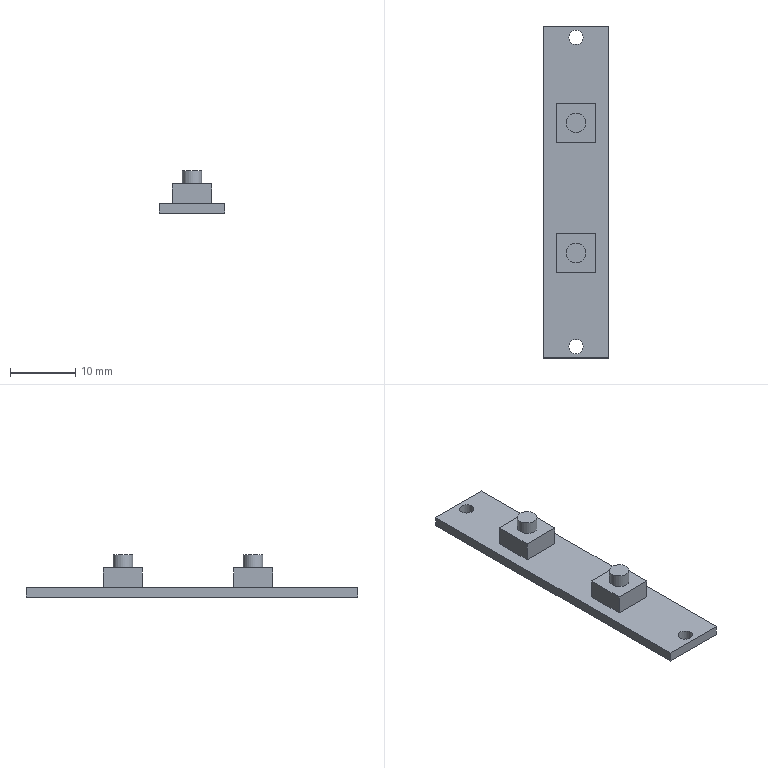Part | STEP file | 1 solid | 22 faces | box 10 x 51 x 6.5 mm | volume 997.87 mm3 | plane 18 | cylinder 4 | commonest cylinder face diameters 2.2 x2 3 x2
STEP:
#1=CARTESIAN_POINT('',(0.,0.,0.));
#2=DIRECTION('',(0.,0.,1.));
#3=DIRECTION('',(1.,0.,0.));
#4=AXIS2_PLACEMENT_3D('',#1,#2,#3);
#5=CARTESIAN_POINT('',(-1.1,12.071,0.));
#6=VERTEX_POINT('',#5);
#7=CARTESIAN_POINT('',(0.,12.071,0.));
#8=DIRECTION('',(0.,0.,-1.));
#9=DIRECTION('',(-1.,0.,0.));
#10=AXIS2_PLACEMENT_3D('',#7,#8,#9);
#11=CIRCLE('',#10,1.1);
#12=CARTESIAN_POINT('',(-5.,-37.179,0.));
#13=DIRECTION('',(0.,0.,1.));
#14=DIRECTION('',(1.,0.,0.));
#15=AXIS2_PLACEMENT_3D('',#12,#13,#14);
#16=PLANE('',#15);
#17=CARTESIAN_POINT('',(3.9,49.25));
#18=CARTESIAN_POINT('',(3.9,51.155));
#19=CARTESIAN_POINT('',(5.55,50.203));
#20=CARTESIAN_POINT('',(7.2,49.25));
#21=CARTESIAN_POINT('',(5.55,48.297));
#22=CARTESIAN_POINT('',(3.9,47.345));
#23=CARTESIAN_POINT('',(3.9,49.25));
#24=(BOUNDED_CURVE()B_SPLINE_CURVE(2,(#17,#18,#19,#20,#21,#22,#23),.UNSPECIFIED.,.T.,.F.)B_SPLINE_CURVE_WITH_KNOTS((1,2,2,2,2,1),(-2.094,0.,2.094,4.189,6.283,8.378),.UNSPECIFIED.)CURVE()GEOMETRIC_REPRESENTATION_ITEM()RATIONAL_B_SPLINE_CURVE((1.,0.5,1.,0.5,1.,0.5,1.))REPRESENTATION_ITEM(''));
#25=(GEOMETRIC_REPRESENTATION_CONTEXT(2)PARAMETRIC_REPRESENTATION_CONTEXT()REPRESENTATION_CONTEXT('',''));
#26=DEFINITIONAL_REPRESENTATION('',(#24),#25);
#27=PCURVE('',#16,#26);
#28=CARTESIAN_POINT('',(0.,12.071,1.5));
#29=DIRECTION('',(0.,0.,-1.));
#30=DIRECTION('',(-1.,0.,0.));
#31=AXIS2_PLACEMENT_3D('',#28,#29,#30);
#32=CYLINDRICAL_SURFACE('',#31,1.1);
#33=CARTESIAN_POINT('',(0.,1.5));
#34=DIRECTION('',(1.,0.));
#35=VECTOR('',#34,1.);
#36=LINE('',#33,#35);
#37=(GEOMETRIC_REPRESENTATION_CONTEXT(2)PARAMETRIC_REPRESENTATION_CONTEXT()REPRESENTATION_CONTEXT('',''));
#38=DEFINITIONAL_REPRESENTATION('',(#36),#37);
#39=PCURVE('',#32,#38);
#40=SURFACE_CURVE('',#11,(#27,#39),.PCURVE_S1.);
#41=EDGE_CURVE('',#6,#6,#40,.T.);
#42=ORIENTED_EDGE('',*,*,#41,.F.);
#43=EDGE_LOOP('',(#42));
#44=FACE_BOUND('',#43,.T.);
#45=CARTESIAN_POINT('',(-1.1,-35.429,0.));
#46=VERTEX_POINT('',#45);
#47=CARTESIAN_POINT('',(0.,-35.429,0.));
#48=DIRECTION('',(0.,0.,-1.));
#49=DIRECTION('',(-1.,0.,0.));
#50=AXIS2_PLACEMENT_3D('',#47,#48,#49);
#51=CIRCLE('',#50,1.1);
#52=CARTESIAN_POINT('',(3.9,1.75));
#53=CARTESIAN_POINT('',(3.9,3.655));
#54=CARTESIAN_POINT('',(5.55,2.703));
#55=CARTESIAN_POINT('',(7.2,1.75));
#56=CARTESIAN_POINT('',(5.55,0.7974));
#57=CARTESIAN_POINT('',(3.9,-0.1553));
#58=CARTESIAN_POINT('',(3.9,1.75));
#59=(BOUNDED_CURVE()B_SPLINE_CURVE(2,(#52,#53,#54,#55,#56,#57,#58),.UNSPECIFIED.,.T.,.F.)B_SPLINE_CURVE_WITH_KNOTS((1,2,2,2,2,1),(-2.094,0.,2.094,4.189,6.283,8.378),.UNSPECIFIED.)CURVE()GEOMETRIC_REPRESENTATION_ITEM()RATIONAL_B_SPLINE_CURVE((1.,0.5,1.,0.5,1.,0.5,1.))REPRESENTATION_ITEM(''));
#60=(GEOMETRIC_REPRESENTATION_CONTEXT(2)PARAMETRIC_REPRESENTATION_CONTEXT()REPRESENTATION_CONTEXT('',''));
#61=DEFINITIONAL_REPRESENTATION('',(#59),#60);
#62=PCURVE('',#16,#61);
#63=CARTESIAN_POINT('',(0.,-35.429,1.5));
#64=DIRECTION('',(0.,0.,-1.));
#65=DIRECTION('',(-1.,0.,0.));
#66=AXIS2_PLACEMENT_3D('',#63,#64,#65);
#67=CYLINDRICAL_SURFACE('',#66,1.1);
#68=CARTESIAN_POINT('',(0.,1.5));
#69=DIRECTION('',(1.,0.));
#70=VECTOR('',#69,1.);
#71=LINE('',#68,#70);
#72=(GEOMETRIC_REPRESENTATION_CONTEXT(2)PARAMETRIC_REPRESENTATION_CONTEXT()REPRESENTATION_CONTEXT('',''));
#73=DEFINITIONAL_REPRESENTATION('',(#71),#72);
#74=PCURVE('',#67,#73);
#75=SURFACE_CURVE('',#51,(#62,#74),.PCURVE_S1.);
#76=EDGE_CURVE('',#46,#46,#75,.T.);
#77=ORIENTED_EDGE('',*,*,#76,.F.);
#78=EDGE_LOOP('',(#77));
#79=FACE_BOUND('',#78,.T.);
#80=CARTESIAN_POINT('',(-5.,13.821,0.));
#81=VERTEX_POINT('',#80);
#82=CARTESIAN_POINT('',(-5.,-37.179,0.));
#83=VERTEX_POINT('',#82);
#84=CARTESIAN_POINT('',(-5.,-37.179,0.));
#85=DIRECTION('',(0.,-1.,0.));
#86=VECTOR('',#85,1.);
#87=LINE('',#84,#86);
#88=CARTESIAN_POINT('',(0.,0.));
#89=DIRECTION('',(0.,-1.));
#90=VECTOR('',#89,1.);
#91=LINE('',#88,#90);
#92=(GEOMETRIC_REPRESENTATION_CONTEXT(2)PARAMETRIC_REPRESENTATION_CONTEXT()REPRESENTATION_CONTEXT('',''));
#93=DEFINITIONAL_REPRESENTATION('',(#91),#92);
#94=PCURVE('',#16,#93);
#95=CARTESIAN_POINT('',(-5.,13.821,1.5));
#96=DIRECTION('',(1.,0.,0.));
#97=DIRECTION('',(0.,0.,-1.));
#98=AXIS2_PLACEMENT_3D('',#95,#96,#97);
#99=PLANE('',#98);
#100=CARTESIAN_POINT('',(1.5,-51.));
#101=DIRECTION('',(0.,-1.));
#102=VECTOR('',#101,1.);
#103=LINE('',#100,#102);
#104=(GEOMETRIC_REPRESENTATION_CONTEXT(2)PARAMETRIC_REPRESENTATION_CONTEXT()REPRESENTATION_CONTEXT('',''));
#105=DEFINITIONAL_REPRESENTATION('',(#103),#104);
#106=PCURVE('',#99,#105);
#107=SURFACE_CURVE('',#87,(#94,#106),.PCURVE_S1.);
#108=EDGE_CURVE('',#81,#83,#107,.T.);
#109=ORIENTED_EDGE('',*,*,#108,.F.);
#110=CARTESIAN_POINT('',(5.,13.821,0.));
#111=VERTEX_POINT('',#110);
#112=CARTESIAN_POINT('',(-5.,13.821,0.));
#113=DIRECTION('',(-1.,0.,0.));
#114=VECTOR('',#113,1.);
#115=LINE('',#112,#114);
#116=CARTESIAN_POINT('',(0.,51.));
#117=DIRECTION('',(-1.,0.));
#118=VECTOR('',#117,1.);
#119=LINE('',#116,#118);
#120=(GEOMETRIC_REPRESENTATION_CONTEXT(2)PARAMETRIC_REPRESENTATION_CONTEXT()REPRESENTATION_CONTEXT('',''));
#121=DEFINITIONAL_REPRESENTATION('',(#119),#120);
#122=PCURVE('',#16,#121);
#123=CARTESIAN_POINT('',(-5.,13.821,1.5));
#124=DIRECTION('',(0.,-1.,0.));
#125=DIRECTION('',(0.,0.,-1.));
#126=AXIS2_PLACEMENT_3D('',#123,#124,#125);
#127=PLANE('',#126);
#128=CARTESIAN_POINT('',(1.5,0.));
#129=DIRECTION('',(0.,-1.));
#130=VECTOR('',#129,1.);
#131=LINE('',#128,#130);
#132=(GEOMETRIC_REPRESENTATION_CONTEXT(2)PARAMETRIC_REPRESENTATION_CONTEXT()REPRESENTATION_CONTEXT('',''));
#133=DEFINITIONAL_REPRESENTATION('',(#131),#132);
#134=PCURVE('',#127,#133);
#135=SURFACE_CURVE('',#115,(#122,#134),.PCURVE_S1.);
#136=EDGE_CURVE('',#111,#81,#135,.T.);
#137=ORIENTED_EDGE('',*,*,#136,.F.);
#138=CARTESIAN_POINT('',(5.,-37.179,0.));
#139=VERTEX_POINT('',#138);
#140=CARTESIAN_POINT('',(5.,-37.179,0.));
#141=DIRECTION('',(0.,1.,0.));
#142=VECTOR('',#141,1.);
#143=LINE('',#140,#142);
#144=CARTESIAN_POINT('',(10.,0.));
#145=DIRECTION('',(0.,1.));
#146=VECTOR('',#145,1.);
#147=LINE('',#144,#146);
#148=(GEOMETRIC_REPRESENTATION_CONTEXT(2)PARAMETRIC_REPRESENTATION_CONTEXT()REPRESENTATION_CONTEXT('',''));
#149=DEFINITIONAL_REPRESENTATION('',(#147),#148);
#150=PCURVE('',#16,#149);
#151=CARTESIAN_POINT('',(5.,13.821,1.5));
#152=DIRECTION('',(-1.,0.,0.));
#153=DIRECTION('',(0.,0.,1.));
#154=AXIS2_PLACEMENT_3D('',#151,#152,#153);
#155=PLANE('',#154);
#156=CARTESIAN_POINT('',(-1.5,-51.));
#157=DIRECTION('',(0.,1.));
#158=VECTOR('',#157,1.);
#159=LINE('',#156,#158);
#160=(GEOMETRIC_REPRESENTATION_CONTEXT(2)PARAMETRIC_REPRESENTATION_CONTEXT()REPRESENTATION_CONTEXT('',''));
#161=DEFINITIONAL_REPRESENTATION('',(#159),#160);
#162=PCURVE('',#155,#161);
#163=SURFACE_CURVE('',#143,(#150,#162),.PCURVE_S1.);
#164=EDGE_CURVE('',#139,#111,#163,.T.);
#165=ORIENTED_EDGE('',*,*,#164,.F.);
#166=CARTESIAN_POINT('',(-5.,-37.179,0.));
#167=DIRECTION('',(1.,0.,0.));
#168=VECTOR('',#167,1.);
#169=LINE('',#166,#168);
#170=CARTESIAN_POINT('',(0.,0.));
#171=DIRECTION('',(1.,0.));
#172=VECTOR('',#171,1.);
#173=LINE('',#170,#172);
#174=(GEOMETRIC_REPRESENTATION_CONTEXT(2)PARAMETRIC_REPRESENTATION_CONTEXT()REPRESENTATION_CONTEXT('',''));
#175=DEFINITIONAL_REPRESENTATION('',(#173),#174);
#176=PCURVE('',#16,#175);
#177=CARTESIAN_POINT('',(-5.,-37.179,1.5));
#178=DIRECTION('',(0.,1.,0.));
#179=DIRECTION('',(0.,0.,1.));
#180=AXIS2_PLACEMENT_3D('',#177,#178,#179);
#181=PLANE('',#180);
#182=CARTESIAN_POINT('',(-1.5,0.));
#183=DIRECTION('',(0.,1.));
#184=VECTOR('',#183,1.);
#185=LINE('',#182,#184);
#186=(GEOMETRIC_REPRESENTATION_CONTEXT(2)PARAMETRIC_REPRESENTATION_CONTEXT()REPRESENTATION_CONTEXT('',''));
#187=DEFINITIONAL_REPRESENTATION('',(#185),#186);
#188=PCURVE('',#181,#187);
#189=SURFACE_CURVE('',#169,(#176,#188),.PCURVE_S1.);
#190=EDGE_CURVE('',#83,#139,#189,.T.);
#191=ORIENTED_EDGE('',*,*,#190,.F.);
#192=EDGE_LOOP('',(#109,#137,#165,#191));
#193=FACE_BOUND('',#192,.T.);
#194=ADVANCED_FACE('',(#44,#79,#193),#16,.F.);
#195=ORIENTED_EDGE('',*,*,#41,.F.);
#196=CARTESIAN_POINT('',(-1.1,12.071,1.5));
#197=VERTEX_POINT('',#196);
#198=CARTESIAN_POINT('',(-1.1,12.071,1.5));
#199=CARTESIAN_POINT('',(-1.1,12.071,0.));
#200=B_SPLINE_CURVE_WITH_KNOTS('',1,(#198,#199),.UNSPECIFIED.,.F.,.F.,(2,2),(0.,1.5),.PIECEWISE_BEZIER_KNOTS.);
#201=CARTESIAN_POINT('',(0.,0.));
#202=DIRECTION('',(0.,1.));
#203=VECTOR('',#202,1.);
#204=LINE('',#201,#203);
#205=(GEOMETRIC_REPRESENTATION_CONTEXT(2)PARAMETRIC_REPRESENTATION_CONTEXT()REPRESENTATION_CONTEXT('',''));
#206=DEFINITIONAL_REPRESENTATION('',(#204),#205);
#207=PCURVE('',#32,#206);
#208=CARTESIAN_POINT('',(6.283,0.));
#209=DIRECTION('',(0.,1.));
#210=VECTOR('',#209,1.);
#211=LINE('',#208,#210);
#212=(GEOMETRIC_REPRESENTATION_CONTEXT(2)PARAMETRIC_REPRESENTATION_CONTEXT()REPRESENTATION_CONTEXT('',''));
#213=DEFINITIONAL_REPRESENTATION('',(#211),#212);
#214=PCURVE('',#32,#213);
#215=SEAM_CURVE('',#200,(#207,#214),.PCURVE_S1.);
#216=EDGE_CURVE('',#197,#6,#215,.T.);
#217=ORIENTED_EDGE('',*,*,#216,.F.);
#218=CARTESIAN_POINT('',(0.,12.071,1.5));
#219=DIRECTION('',(0.,0.,-1.));
#220=DIRECTION('',(-1.,0.,0.));
#221=AXIS2_PLACEMENT_3D('',#218,#219,#220);
#222=CIRCLE('',#221,1.1);
#223=CARTESIAN_POINT('',(0.,0.));
#224=DIRECTION('',(1.,0.));
#225=VECTOR('',#224,1.);
#226=LINE('',#223,#225);
#227=(GEOMETRIC_REPRESENTATION_CONTEXT(2)PARAMETRIC_REPRESENTATION_CONTEXT()REPRESENTATION_CONTEXT('',''));
#228=DEFINITIONAL_REPRESENTATION('',(#226),#227);
#229=PCURVE('',#32,#228);
#230=CARTESIAN_POINT('',(-5.,-37.179,1.5));
#231=DIRECTION('',(0.,0.,1.));
#232=DIRECTION('',(1.,0.,0.));
#233=AXIS2_PLACEMENT_3D('',#230,#231,#232);
#234=PLANE('',#233);
#235=CARTESIAN_POINT('',(3.9,49.25));
#236=CARTESIAN_POINT('',(3.9,51.155));
#237=CARTESIAN_POINT('',(5.55,50.203));
#238=CARTESIAN_POINT('',(7.2,49.25));
#239=CARTESIAN_POINT('',(5.55,48.297));
#240=CARTESIAN_POINT('',(3.9,47.345));
#241=CARTESIAN_POINT('',(3.9,49.25));
#242=(BOUNDED_CURVE()B_SPLINE_CURVE(2,(#235,#236,#237,#238,#239,#240,#241),.UNSPECIFIED.,.T.,.F.)B_SPLINE_CURVE_WITH_KNOTS((1,2,2,2,2,1),(-2.094,0.,2.094,4.189,6.283,8.378),.UNSPECIFIED.)CURVE()GEOMETRIC_REPRESENTATION_ITEM()RATIONAL_B_SPLINE_CURVE((1.,0.5,1.,0.5,1.,0.5,1.))REPRESENTATION_ITEM(''));
#243=(GEOMETRIC_REPRESENTATION_CONTEXT(2)PARAMETRIC_REPRESENTATION_CONTEXT()REPRESENTATION_CONTEXT('',''));
#244=DEFINITIONAL_REPRESENTATION('',(#242),#243);
#245=PCURVE('',#234,#244);
#246=SURFACE_CURVE('',#222,(#229,#245),.PCURVE_S1.);
#247=EDGE_CURVE('',#197,#197,#246,.T.);
#248=ORIENTED_EDGE('',*,*,#247,.T.);
#249=ORIENTED_EDGE('',*,*,#216,.T.);
#250=EDGE_LOOP('',(#195,#217,#248,#249));
#251=FACE_BOUND('',#250,.F.);
#252=ADVANCED_FACE('',(#251),#32,.F.);
#253=ORIENTED_EDGE('',*,*,#76,.F.);
#254=CARTESIAN_POINT('',(-1.1,-35.429,1.5));
#255=VERTEX_POINT('',#254);
#256=CARTESIAN_POINT('',(-1.1,-35.429,1.5));
#257=CARTESIAN_POINT('',(-1.1,-35.429,0.));
#258=B_SPLINE_CURVE_WITH_KNOTS('',1,(#256,#257),.UNSPECIFIED.,.F.,.F.,(2,2),(0.,1.5),.PIECEWISE_BEZIER_KNOTS.);
#259=CARTESIAN_POINT('',(0.,0.));
#260=DIRECTION('',(0.,1.));
#261=VECTOR('',#260,1.);
#262=LINE('',#259,#261);
#263=(GEOMETRIC_REPRESENTATION_CONTEXT(2)PARAMETRIC_REPRESENTATION_CONTEXT()REPRESENTATION_CONTEXT('',''));
#264=DEFINITIONAL_REPRESENTATION('',(#262),#263);
#265=PCURVE('',#67,#264);
#266=CARTESIAN_POINT('',(6.283,0.));
#267=DIRECTION('',(0.,1.));
#268=VECTOR('',#267,1.);
#269=LINE('',#266,#268);
#270=(GEOMETRIC_REPRESENTATION_CONTEXT(2)PARAMETRIC_REPRESENTATION_CONTEXT()REPRESENTATION_CONTEXT('',''));
#271=DEFINITIONAL_REPRESENTATION('',(#269),#270);
#272=PCURVE('',#67,#271);
#273=SEAM_CURVE('',#258,(#265,#272),.PCURVE_S1.);
#274=EDGE_CURVE('',#255,#46,#273,.T.);
#275=ORIENTED_EDGE('',*,*,#274,.F.);
#276=CARTESIAN_POINT('',(0.,-35.429,1.5));
#277=DIRECTION('',(0.,0.,-1.));
#278=DIRECTION('',(-1.,0.,0.));
#279=AXIS2_PLACEMENT_3D('',#276,#277,#278);
#280=CIRCLE('',#279,1.1);
#281=CARTESIAN_POINT('',(0.,0.));
#282=DIRECTION('',(1.,0.));
#283=VECTOR('',#282,1.);
#284=LINE('',#281,#283);
#285=(GEOMETRIC_REPRESENTATION_CONTEXT(2)PARAMETRIC_REPRESENTATION_CONTEXT()REPRESENTATION_CONTEXT('',''));
#286=DEFINITIONAL_REPRESENTATION('',(#284),#285);
#287=PCURVE('',#67,#286);
#288=CARTESIAN_POINT('',(3.9,1.75));
#289=CARTESIAN_POINT('',(3.9,3.655));
#290=CARTESIAN_POINT('',(5.55,2.703));
#291=CARTESIAN_POINT('',(7.2,1.75));
#292=CARTESIAN_POINT('',(5.55,0.7974));
#293=CARTESIAN_POINT('',(3.9,-0.1553));
#294=CARTESIAN_POINT('',(3.9,1.75));
#295=(BOUNDED_CURVE()B_SPLINE_CURVE(2,(#288,#289,#290,#291,#292,#293,#294),.UNSPECIFIED.,.T.,.F.)B_SPLINE_CURVE_WITH_KNOTS((1,2,2,2,2,1),(-2.094,0.,2.094,4.189,6.283,8.378),.UNSPECIFIED.)CURVE()GEOMETRIC_REPRESENTATION_ITEM()RATIONAL_B_SPLINE_CURVE((1.,0.5,1.,0.5,1.,0.5,1.))REPRESENTATION_ITEM(''));
#296=(GEOMETRIC_REPRESENTATION_CONTEXT(2)PARAMETRIC_REPRESENTATION_CONTEXT()REPRESENTATION_CONTEXT('',''));
#297=DEFINITIONAL_REPRESENTATION('',(#295),#296);
#298=PCURVE('',#234,#297);
#299=SURFACE_CURVE('',#280,(#287,#298),.PCURVE_S1.);
#300=EDGE_CURVE('',#255,#255,#299,.T.);
#301=ORIENTED_EDGE('',*,*,#300,.T.);
#302=ORIENTED_EDGE('',*,*,#274,.T.);
#303=EDGE_LOOP('',(#253,#275,#301,#302));
#304=FACE_BOUND('',#303,.F.);
#305=ADVANCED_FACE('',(#304),#67,.F.);
#306=ORIENTED_EDGE('',*,*,#190,.T.);
#307=CARTESIAN_POINT('',(5.,-37.179,1.5));
#308=VERTEX_POINT('',#307);
#309=CARTESIAN_POINT('',(5.,-37.179,1.5));
#310=DIRECTION('',(0.,0.,-1.));
#311=VECTOR('',#310,1.);
#312=LINE('',#309,#311);
#313=CARTESIAN_POINT('',(0.,10.));
#314=DIRECTION('',(-1.,0.));
#315=VECTOR('',#314,1.);
#316=LINE('',#313,#315);
#317=(GEOMETRIC_REPRESENTATION_CONTEXT(2)PARAMETRIC_REPRESENTATION_CONTEXT()REPRESENTATION_CONTEXT('',''));
#318=DEFINITIONAL_REPRESENTATION('',(#316),#317);
#319=PCURVE('',#181,#318);
#320=CARTESIAN_POINT('',(0.,-51.));
#321=DIRECTION('',(-1.,0.));
#322=VECTOR('',#321,1.);
#323=LINE('',#320,#322);
#324=(GEOMETRIC_REPRESENTATION_CONTEXT(2)PARAMETRIC_REPRESENTATION_CONTEXT()REPRESENTATION_CONTEXT('',''));
#325=DEFINITIONAL_REPRESENTATION('',(#323),#324);
#326=PCURVE('',#155,#325);
#327=SURFACE_CURVE('',#312,(#319,#326),.PCURVE_S1.);
#328=EDGE_CURVE('',#308,#139,#327,.T.);
#329=ORIENTED_EDGE('',*,*,#328,.F.);
#330=CARTESIAN_POINT('',(-5.,-37.179,1.5));
#331=VERTEX_POINT('',#330);
#332=CARTESIAN_POINT('',(-5.,-37.179,1.5));
#333=DIRECTION('',(1.,0.,0.));
#334=VECTOR('',#333,1.);
#335=LINE('',#332,#334);
#336=CARTESIAN_POINT('',(0.,0.));
#337=DIRECTION('',(0.,1.));
#338=VECTOR('',#337,1.);
#339=LINE('',#336,#338);
#340=(GEOMETRIC_REPRESENTATION_CONTEXT(2)PARAMETRIC_REPRESENTATION_CONTEXT()REPRESENTATION_CONTEXT('',''));
#341=DEFINITIONAL_REPRESENTATION('',(#339),#340);
#342=PCURVE('',#181,#341);
#343=CARTESIAN_POINT('',(0.,0.));
#344=DIRECTION('',(1.,0.));
#345=VECTOR('',#344,1.);
#346=LINE('',#343,#345);
#347=(GEOMETRIC_REPRESENTATION_CONTEXT(2)PARAMETRIC_REPRESENTATION_CONTEXT()REPRESENTATION_CONTEXT('',''));
#348=DEFINITIONAL_REPRESENTATION('',(#346),#347);
#349=PCURVE('',#234,#348);
#350=SURFACE_CURVE('',#335,(#342,#349),.PCURVE_S1.);
#351=EDGE_CURVE('',#331,#308,#350,.T.);
#352=ORIENTED_EDGE('',*,*,#351,.F.);
#353=CARTESIAN_POINT('',(-5.,-37.179,1.5));
#354=DIRECTION('',(0.,0.,1.));
#355=VECTOR('',#354,1.);
#356=LINE('',#353,#355);
#357=CARTESIAN_POINT('',(0.,0.));
#358=DIRECTION('',(1.,0.));
#359=VECTOR('',#358,1.);
#360=LINE('',#357,#359);
#361=(GEOMETRIC_REPRESENTATION_CONTEXT(2)PARAMETRIC_REPRESENTATION_CONTEXT()REPRESENTATION_CONTEXT('',''));
#362=DEFINITIONAL_REPRESENTATION('',(#360),#361);
#363=PCURVE('',#181,#362);
#364=CARTESIAN_POINT('',(0.,-51.));
#365=DIRECTION('',(-1.,0.));
#366=VECTOR('',#365,1.);
#367=LINE('',#364,#366);
#368=(GEOMETRIC_REPRESENTATION_CONTEXT(2)PARAMETRIC_REPRESENTATION_CONTEXT()REPRESENTATION_CONTEXT('',''));
#369=DEFINITIONAL_REPRESENTATION('',(#367),#368);
#370=PCURVE('',#99,#369);
#371=SURFACE_CURVE('',#356,(#363,#370),.PCURVE_S1.);
#372=EDGE_CURVE('',#83,#331,#371,.T.);
#373=ORIENTED_EDGE('',*,*,#372,.F.);
#374=EDGE_LOOP('',(#306,#329,#352,#373));
#375=FACE_BOUND('',#374,.T.);
#376=ADVANCED_FACE('',(#375),#181,.F.);
#377=ORIENTED_EDGE('',*,*,#108,.T.);
#378=ORIENTED_EDGE('',*,*,#372,.T.);
#379=CARTESIAN_POINT('',(-5.,13.821,1.5));
#380=VERTEX_POINT('',#379);
#381=CARTESIAN_POINT('',(-5.,13.821,1.5));
#382=DIRECTION('',(0.,-1.,0.));
#383=VECTOR('',#382,1.);
#384=LINE('',#381,#383);
#385=CARTESIAN_POINT('',(0.,0.));
#386=DIRECTION('',(0.,-1.));
#387=VECTOR('',#386,1.);
#388=LINE('',#385,#387);
#389=(GEOMETRIC_REPRESENTATION_CONTEXT(2)PARAMETRIC_REPRESENTATION_CONTEXT()REPRESENTATION_CONTEXT('',''));
#390=DEFINITIONAL_REPRESENTATION('',(#388),#389);
#391=PCURVE('',#99,#390);
#392=CARTESIAN_POINT('',(0.,51.));
#393=DIRECTION('',(0.,-1.));
#394=VECTOR('',#393,1.);
#395=LINE('',#392,#394);
#396=(GEOMETRIC_REPRESENTATION_CONTEXT(2)PARAMETRIC_REPRESENTATION_CONTEXT()REPRESENTATION_CONTEXT('',''));
#397=DEFINITIONAL_REPRESENTATION('',(#395),#396);
#398=PCURVE('',#234,#397);
#399=SURFACE_CURVE('',#384,(#391,#398),.PCURVE_S1.);
#400=EDGE_CURVE('',#380,#331,#399,.T.);
#401=ORIENTED_EDGE('',*,*,#400,.F.);
#402=CARTESIAN_POINT('',(-5.,13.821,1.5));
#403=DIRECTION('',(0.,0.,1.));
#404=VECTOR('',#403,1.);
#405=LINE('',#402,#404);
#406=CARTESIAN_POINT('',(0.,0.));
#407=DIRECTION('',(-1.,0.));
#408=VECTOR('',#407,1.);
#409=LINE('',#406,#408);
#410=(GEOMETRIC_REPRESENTATION_CONTEXT(2)PARAMETRIC_REPRESENTATION_CONTEXT()REPRESENTATION_CONTEXT('',''));
#411=DEFINITIONAL_REPRESENTATION('',(#409),#410);
#412=PCURVE('',#99,#411);
#413=CARTESIAN_POINT('',(0.,0.));
#414=DIRECTION('',(-1.,0.));
#415=VECTOR('',#414,1.);
#416=LINE('',#413,#415);
#417=(GEOMETRIC_REPRESENTATION_CONTEXT(2)PARAMETRIC_REPRESENTATION_CONTEXT()REPRESENTATION_CONTEXT('',''));
#418=DEFINITIONAL_REPRESENTATION('',(#416),#417);
#419=PCURVE('',#127,#418);
#420=SURFACE_CURVE('',#405,(#412,#419),.PCURVE_S1.);
#421=EDGE_CURVE('',#81,#380,#420,.T.);
#422=ORIENTED_EDGE('',*,*,#421,.F.);
#423=EDGE_LOOP('',(#377,#378,#401,#422));
#424=FACE_BOUND('',#423,.T.);
#425=ADVANCED_FACE('',(#424),#99,.F.);
#426=ORIENTED_EDGE('',*,*,#136,.T.);
#427=ORIENTED_EDGE('',*,*,#421,.T.);
#428=CARTESIAN_POINT('',(5.,13.821,1.5));
#429=VERTEX_POINT('',#428);
#430=CARTESIAN_POINT('',(-5.,13.821,1.5));
#431=DIRECTION('',(-1.,0.,0.));
#432=VECTOR('',#431,1.);
#433=LINE('',#430,#432);
#434=CARTESIAN_POINT('',(0.,0.));
#435=DIRECTION('',(0.,-1.));
#436=VECTOR('',#435,1.);
#437=LINE('',#434,#436);
#438=(GEOMETRIC_REPRESENTATION_CONTEXT(2)PARAMETRIC_REPRESENTATION_CONTEXT()REPRESENTATION_CONTEXT('',''));
#439=DEFINITIONAL_REPRESENTATION('',(#437),#438);
#440=PCURVE('',#127,#439);
#441=CARTESIAN_POINT('',(0.,51.));
#442=DIRECTION('',(-1.,0.));
#443=VECTOR('',#442,1.);
#444=LINE('',#441,#443);
#445=(GEOMETRIC_REPRESENTATION_CONTEXT(2)PARAMETRIC_REPRESENTATION_CONTEXT()REPRESENTATION_CONTEXT('',''));
#446=DEFINITIONAL_REPRESENTATION('',(#444),#445);
#447=PCURVE('',#234,#446);
#448=SURFACE_CURVE('',#433,(#440,#447),.PCURVE_S1.);
#449=EDGE_CURVE('',#429,#380,#448,.T.);
#450=ORIENTED_EDGE('',*,*,#449,.F.);
#451=CARTESIAN_POINT('',(5.,13.821,1.5));
#452=DIRECTION('',(0.,0.,1.));
#453=VECTOR('',#452,1.);
#454=LINE('',#451,#453);
#455=CARTESIAN_POINT('',(0.,10.));
#456=DIRECTION('',(-1.,0.));
#457=VECTOR('',#456,1.);
#458=LINE('',#455,#457);
#459=(GEOMETRIC_REPRESENTATION_CONTEXT(2)PARAMETRIC_REPRESENTATION_CONTEXT()REPRESENTATION_CONTEXT('',''));
#460=DEFINITIONAL_REPRESENTATION('',(#458),#459);
#461=PCURVE('',#127,#460);
#462=CARTESIAN_POINT('',(0.,0.));
#463=DIRECTION('',(1.,0.));
#464=VECTOR('',#463,1.);
#465=LINE('',#462,#464);
#466=(GEOMETRIC_REPRESENTATION_CONTEXT(2)PARAMETRIC_REPRESENTATION_CONTEXT()REPRESENTATION_CONTEXT('',''));
#467=DEFINITIONAL_REPRESENTATION('',(#465),#466);
#468=PCURVE('',#155,#467);
#469=SURFACE_CURVE('',#454,(#461,#468),.PCURVE_S1.);
#470=EDGE_CURVE('',#111,#429,#469,.T.);
#471=ORIENTED_EDGE('',*,*,#470,.F.);
#472=EDGE_LOOP('',(#426,#427,#450,#471));
#473=FACE_BOUND('',#472,.T.);
#474=ADVANCED_FACE('',(#473),#127,.F.);
#475=ORIENTED_EDGE('',*,*,#164,.T.);
#476=ORIENTED_EDGE('',*,*,#470,.T.);
#477=CARTESIAN_POINT('',(5.,13.821,1.5));
#478=DIRECTION('',(0.,1.,0.));
#479=VECTOR('',#478,1.);
#480=LINE('',#477,#479);
#481=CARTESIAN_POINT('',(0.,0.));
#482=DIRECTION('',(0.,1.));
#483=VECTOR('',#482,1.);
#484=LINE('',#481,#483);
#485=(GEOMETRIC_REPRESENTATION_CONTEXT(2)PARAMETRIC_REPRESENTATION_CONTEXT()REPRESENTATION_CONTEXT('',''));
#486=DEFINITIONAL_REPRESENTATION('',(#484),#485);
#487=PCURVE('',#155,#486);
#488=CARTESIAN_POINT('',(10.,51.));
#489=DIRECTION('',(0.,1.));
#490=VECTOR('',#489,1.);
#491=LINE('',#488,#490);
#492=(GEOMETRIC_REPRESENTATION_CONTEXT(2)PARAMETRIC_REPRESENTATION_CONTEXT()REPRESENTATION_CONTEXT('',''));
#493=DEFINITIONAL_REPRESENTATION('',(#491),#492);
#494=PCURVE('',#234,#493);
#495=SURFACE_CURVE('',#480,(#487,#494),.PCURVE_S1.);
#496=EDGE_CURVE('',#308,#429,#495,.T.);
#497=ORIENTED_EDGE('',*,*,#496,.F.);
#498=ORIENTED_EDGE('',*,*,#328,.T.);
#499=EDGE_LOOP('',(#475,#476,#497,#498));
#500=FACE_BOUND('',#499,.T.);
#501=ADVANCED_FACE('',(#500),#155,.F.);
#502=CARTESIAN_POINT('',(-3.,1.941,1.5));
#503=VERTEX_POINT('',#502);
#504=CARTESIAN_POINT('',(3.,1.941,1.5));
#505=VERTEX_POINT('',#504);
#506=CARTESIAN_POINT('',(-5.,1.941,1.5));
#507=DIRECTION('',(1.,0.,0.));
#508=VECTOR('',#507,1.);
#509=LINE('',#506,#508);
#510=CARTESIAN_POINT('',(0.,39.12));
#511=DIRECTION('',(1.,0.));
#512=VECTOR('',#511,1.);
#513=LINE('',#510,#512);
#514=(GEOMETRIC_REPRESENTATION_CONTEXT(2)PARAMETRIC_REPRESENTATION_CONTEXT()REPRESENTATION_CONTEXT('',''));
#515=DEFINITIONAL_REPRESENTATION('',(#513),#514);
#516=PCURVE('',#234,#515);
#517=CARTESIAN_POINT('',(-3.,1.941,4.5));
#518=DIRECTION('',(0.,-1.,0.));
#519=DIRECTION('',(0.,0.,-1.));
#520=AXIS2_PLACEMENT_3D('',#517,#518,#519);
#521=PLANE('',#520);
#522=CARTESIAN_POINT('',(3.,-2.));
#523=DIRECTION('',(0.,1.));
#524=VECTOR('',#523,1.);
#525=LINE('',#522,#524);
#526=(GEOMETRIC_REPRESENTATION_CONTEXT(2)PARAMETRIC_REPRESENTATION_CONTEXT()REPRESENTATION_CONTEXT('',''));
#527=DEFINITIONAL_REPRESENTATION('',(#525),#526);
#528=PCURVE('',#521,#527);
#529=SURFACE_CURVE('',#509,(#516,#528),.PCURVE_S1.);
#530=EDGE_CURVE('',#503,#505,#529,.T.);
#531=ORIENTED_EDGE('',*,*,#530,.T.);
#532=CARTESIAN_POINT('',(3.,-4.059,1.5));
#533=VERTEX_POINT('',#532);
#534=CARTESIAN_POINT('',(3.,-37.179,1.5));
#535=DIRECTION('',(0.,-1.,0.));
#536=VECTOR('',#535,1.);
#537=LINE('',#534,#536);
#538=CARTESIAN_POINT('',(8.,0.));
#539=DIRECTION('',(0.,-1.));
#540=VECTOR('',#539,1.);
#541=LINE('',#538,#540);
#542=(GEOMETRIC_REPRESENTATION_CONTEXT(2)PARAMETRIC_REPRESENTATION_CONTEXT()REPRESENTATION_CONTEXT('',''));
#543=DEFINITIONAL_REPRESENTATION('',(#541),#542);
#544=PCURVE('',#234,#543);
#545=CARTESIAN_POINT('',(3.,1.941,4.5));
#546=DIRECTION('',(-1.,0.,0.));
#547=DIRECTION('',(0.,0.,1.));
#548=AXIS2_PLACEMENT_3D('',#545,#546,#547);
#549=PLANE('',#548);
#550=CARTESIAN_POINT('',(-3.,-39.12));
#551=DIRECTION('',(0.,-1.));
#552=VECTOR('',#551,1.);
#553=LINE('',#550,#552);
#554=(GEOMETRIC_REPRESENTATION_CONTEXT(2)PARAMETRIC_REPRESENTATION_CONTEXT()REPRESENTATION_CONTEXT('',''));
#555=DEFINITIONAL_REPRESENTATION('',(#553),#554);
#556=PCURVE('',#549,#555);
#557=SURFACE_CURVE('',#537,(#544,#556),.PCURVE_S1.);
#558=EDGE_CURVE('',#505,#533,#557,.T.);
#559=ORIENTED_EDGE('',*,*,#558,.T.);
#560=CARTESIAN_POINT('',(-3.,-4.059,1.5));
#561=VERTEX_POINT('',#560);
#562=CARTESIAN_POINT('',(-5.,-4.059,1.5));
#563=DIRECTION('',(-1.,0.,0.));
#564=VECTOR('',#563,1.);
#565=LINE('',#562,#564);
#566=CARTESIAN_POINT('',(0.,33.12));
#567=DIRECTION('',(-1.,0.));
#568=VECTOR('',#567,1.);
#569=LINE('',#566,#568);
#570=(GEOMETRIC_REPRESENTATION_CONTEXT(2)PARAMETRIC_REPRESENTATION_CONTEXT()REPRESENTATION_CONTEXT('',''));
#571=DEFINITIONAL_REPRESENTATION('',(#569),#570);
#572=PCURVE('',#234,#571);
#573=CARTESIAN_POINT('',(-3.,-4.059,4.5));
#574=DIRECTION('',(0.,1.,0.));
#575=DIRECTION('',(0.,0.,1.));
#576=AXIS2_PLACEMENT_3D('',#573,#574,#575);
#577=PLANE('',#576);
#578=CARTESIAN_POINT('',(-3.,-2.));
#579=DIRECTION('',(0.,-1.));
#580=VECTOR('',#579,1.);
#581=LINE('',#578,#580);
#582=(GEOMETRIC_REPRESENTATION_CONTEXT(2)PARAMETRIC_REPRESENTATION_CONTEXT()REPRESENTATION_CONTEXT('',''));
#583=DEFINITIONAL_REPRESENTATION('',(#581),#582);
#584=PCURVE('',#577,#583);
#585=SURFACE_CURVE('',#565,(#572,#584),.PCURVE_S1.);
#586=EDGE_CURVE('',#533,#561,#585,.T.);
#587=ORIENTED_EDGE('',*,*,#586,.T.);
#588=CARTESIAN_POINT('',(-3.,-37.179,1.5));
#589=DIRECTION('',(0.,1.,0.));
#590=VECTOR('',#589,1.);
#591=LINE('',#588,#590);
#592=CARTESIAN_POINT('',(2.,0.));
#593=DIRECTION('',(0.,1.));
#594=VECTOR('',#593,1.);
#595=LINE('',#592,#594);
#596=(GEOMETRIC_REPRESENTATION_CONTEXT(2)PARAMETRIC_REPRESENTATION_CONTEXT()REPRESENTATION_CONTEXT('',''));
#597=DEFINITIONAL_REPRESENTATION('',(#595),#596);
#598=PCURVE('',#234,#597);
#599=CARTESIAN_POINT('',(-3.,1.941,4.5));
#600=DIRECTION('',(1.,0.,0.));
#601=DIRECTION('',(0.,0.,-1.));
#602=AXIS2_PLACEMENT_3D('',#599,#600,#601);
#603=PLANE('',#602);
#604=CARTESIAN_POINT('',(3.,-39.12));
#605=DIRECTION('',(0.,1.));
#606=VECTOR('',#605,1.);
#607=LINE('',#604,#606);
#608=(GEOMETRIC_REPRESENTATION_CONTEXT(2)PARAMETRIC_REPRESENTATION_CONTEXT()REPRESENTATION_CONTEXT('',''));
#609=DEFINITIONAL_REPRESENTATION('',(#607),#608);
#610=PCURVE('',#603,#609);
#611=SURFACE_CURVE('',#591,(#598,#610),.PCURVE_S1.);
#612=EDGE_CURVE('',#561,#503,#611,.T.);
#613=ORIENTED_EDGE('',*,*,#612,.T.);
#614=EDGE_LOOP('',(#531,#559,#587,#613));
#615=FACE_BOUND('',#614,.T.);
#616=ORIENTED_EDGE('',*,*,#247,.T.);
#617=EDGE_LOOP('',(#616));
#618=FACE_BOUND('',#617,.T.);
#619=ORIENTED_EDGE('',*,*,#300,.T.);
#620=EDGE_LOOP('',(#619));
#621=FACE_BOUND('',#620,.T.);
#622=CARTESIAN_POINT('',(-3.,-18.059,1.5));
#623=VERTEX_POINT('',#622);
#624=CARTESIAN_POINT('',(3.,-18.059,1.5));
#625=VERTEX_POINT('',#624);
#626=CARTESIAN_POINT('',(-5.,-18.059,1.5));
#627=DIRECTION('',(1.,0.,0.));
#628=VECTOR('',#627,1.);
#629=LINE('',#626,#628);
#630=CARTESIAN_POINT('',(0.,19.12));
#631=DIRECTION('',(1.,0.));
#632=VECTOR('',#631,1.);
#633=LINE('',#630,#632);
#634=(GEOMETRIC_REPRESENTATION_CONTEXT(2)PARAMETRIC_REPRESENTATION_CONTEXT()REPRESENTATION_CONTEXT('',''));
#635=DEFINITIONAL_REPRESENTATION('',(#633),#634);
#636=PCURVE('',#234,#635);
#637=CARTESIAN_POINT('',(-3.,-18.059,4.5));
#638=DIRECTION('',(0.,-1.,0.));
#639=DIRECTION('',(0.,0.,-1.));
#640=AXIS2_PLACEMENT_3D('',#637,#638,#639);
#641=PLANE('',#640);
#642=CARTESIAN_POINT('',(3.,-2.));
#643=DIRECTION('',(0.,1.));
#644=VECTOR('',#643,1.);
#645=LINE('',#642,#644);
#646=(GEOMETRIC_REPRESENTATION_CONTEXT(2)PARAMETRIC_REPRESENTATION_CONTEXT()REPRESENTATION_CONTEXT('',''));
#647=DEFINITIONAL_REPRESENTATION('',(#645),#646);
#648=PCURVE('',#641,#647);
#649=SURFACE_CURVE('',#629,(#636,#648),.PCURVE_S1.);
#650=EDGE_CURVE('',#623,#625,#649,.T.);
#651=ORIENTED_EDGE('',*,*,#650,.T.);
#652=CARTESIAN_POINT('',(3.,-24.059,1.5));
#653=VERTEX_POINT('',#652);
#654=CARTESIAN_POINT('',(3.,-37.179,1.5));
#655=DIRECTION('',(0.,-1.,0.));
#656=VECTOR('',#655,1.);
#657=LINE('',#654,#656);
#658=CARTESIAN_POINT('',(8.,0.));
#659=DIRECTION('',(0.,-1.));
#660=VECTOR('',#659,1.);
#661=LINE('',#658,#660);
#662=(GEOMETRIC_REPRESENTATION_CONTEXT(2)PARAMETRIC_REPRESENTATION_CONTEXT()REPRESENTATION_CONTEXT('',''));
#663=DEFINITIONAL_REPRESENTATION('',(#661),#662);
#664=PCURVE('',#234,#663);
#665=CARTESIAN_POINT('',(3.,-18.059,4.5));
#666=DIRECTION('',(-1.,0.,0.));
#667=DIRECTION('',(0.,0.,1.));
#668=AXIS2_PLACEMENT_3D('',#665,#666,#667);
#669=PLANE('',#668);
#670=CARTESIAN_POINT('',(-3.,-19.12));
#671=DIRECTION('',(0.,-1.));
#672=VECTOR('',#671,1.);
#673=LINE('',#670,#672);
#674=(GEOMETRIC_REPRESENTATION_CONTEXT(2)PARAMETRIC_REPRESENTATION_CONTEXT()REPRESENTATION_CONTEXT('',''));
#675=DEFINITIONAL_REPRESENTATION('',(#673),#674);
#676=PCURVE('',#669,#675);
#677=SURFACE_CURVE('',#657,(#664,#676),.PCURVE_S1.);
#678=EDGE_CURVE('',#625,#653,#677,.T.);
#679=ORIENTED_EDGE('',*,*,#678,.T.);
#680=CARTESIAN_POINT('',(-3.,-24.059,1.5));
#681=VERTEX_POINT('',#680);
#682=CARTESIAN_POINT('',(-5.,-24.059,1.5));
#683=DIRECTION('',(-1.,0.,0.));
#684=VECTOR('',#683,1.);
#685=LINE('',#682,#684);
#686=CARTESIAN_POINT('',(0.,13.12));
#687=DIRECTION('',(-1.,0.));
#688=VECTOR('',#687,1.);
#689=LINE('',#686,#688);
#690=(GEOMETRIC_REPRESENTATION_CONTEXT(2)PARAMETRIC_REPRESENTATION_CONTEXT()REPRESENTATION_CONTEXT('',''));
#691=DEFINITIONAL_REPRESENTATION('',(#689),#690);
#692=PCURVE('',#234,#691);
#693=CARTESIAN_POINT('',(-3.,-24.059,4.5));
#694=DIRECTION('',(0.,1.,0.));
#695=DIRECTION('',(0.,0.,1.));
#696=AXIS2_PLACEMENT_3D('',#693,#694,#695);
#697=PLANE('',#696);
#698=CARTESIAN_POINT('',(-3.,-2.));
#699=DIRECTION('',(0.,-1.));
#700=VECTOR('',#699,1.);
#701=LINE('',#698,#700);
#702=(GEOMETRIC_REPRESENTATION_CONTEXT(2)PARAMETRIC_REPRESENTATION_CONTEXT()REPRESENTATION_CONTEXT('',''));
#703=DEFINITIONAL_REPRESENTATION('',(#701),#702);
#704=PCURVE('',#697,#703);
#705=SURFACE_CURVE('',#685,(#692,#704),.PCURVE_S1.);
#706=EDGE_CURVE('',#653,#681,#705,.T.);
#707=ORIENTED_EDGE('',*,*,#706,.T.);
#708=CARTESIAN_POINT('',(-3.,-37.179,1.5));
#709=DIRECTION('',(0.,1.,0.));
#710=VECTOR('',#709,1.);
#711=LINE('',#708,#710);
#712=CARTESIAN_POINT('',(2.,0.));
#713=DIRECTION('',(0.,1.));
#714=VECTOR('',#713,1.);
#715=LINE('',#712,#714);
#716=(GEOMETRIC_REPRESENTATION_CONTEXT(2)PARAMETRIC_REPRESENTATION_CONTEXT()REPRESENTATION_CONTEXT('',''));
#717=DEFINITIONAL_REPRESENTATION('',(#715),#716);
#718=PCURVE('',#234,#717);
#719=CARTESIAN_POINT('',(-3.,-18.059,4.5));
#720=DIRECTION('',(1.,0.,0.));
#721=DIRECTION('',(0.,0.,-1.));
#722=AXIS2_PLACEMENT_3D('',#719,#720,#721);
#723=PLANE('',#722);
#724=CARTESIAN_POINT('',(3.,-19.12));
#725=DIRECTION('',(0.,1.));
#726=VECTOR('',#725,1.);
#727=LINE('',#724,#726);
#728=(GEOMETRIC_REPRESENTATION_CONTEXT(2)PARAMETRIC_REPRESENTATION_CONTEXT()REPRESENTATION_CONTEXT('',''));
#729=DEFINITIONAL_REPRESENTATION('',(#727),#728);
#730=PCURVE('',#723,#729);
#731=SURFACE_CURVE('',#711,(#718,#730),.PCURVE_S1.);
#732=EDGE_CURVE('',#681,#623,#731,.T.);
#733=ORIENTED_EDGE('',*,*,#732,.T.);
#734=EDGE_LOOP('',(#651,#679,#707,#733));
#735=FACE_BOUND('',#734,.T.);
#736=ORIENTED_EDGE('',*,*,#496,.T.);
#737=ORIENTED_EDGE('',*,*,#449,.T.);
#738=ORIENTED_EDGE('',*,*,#400,.T.);
#739=ORIENTED_EDGE('',*,*,#351,.T.);
#740=EDGE_LOOP('',(#736,#737,#738,#739));
#741=FACE_BOUND('',#740,.T.);
#742=ADVANCED_FACE('',(#615,#618,#621,#735,#741),#234,.T.);
#743=ORIENTED_EDGE('',*,*,#558,.F.);
#744=CARTESIAN_POINT('',(3.,1.941,4.5));
#745=VERTEX_POINT('',#744);
#746=CARTESIAN_POINT('',(3.,1.941,4.5));
#747=DIRECTION('',(0.,0.,-1.));
#748=VECTOR('',#747,1.);
#749=LINE('',#746,#748);
#750=CARTESIAN_POINT('',(0.,0.));
#751=DIRECTION('',(-1.,0.));
#752=VECTOR('',#751,1.);
#753=LINE('',#750,#752);
#754=(GEOMETRIC_REPRESENTATION_CONTEXT(2)PARAMETRIC_REPRESENTATION_CONTEXT()REPRESENTATION_CONTEXT('',''));
#755=DEFINITIONAL_REPRESENTATION('',(#753),#754);
#756=PCURVE('',#549,#755);
#757=CARTESIAN_POINT('',(0.,6.));
#758=DIRECTION('',(1.,0.));
#759=VECTOR('',#758,1.);
#760=LINE('',#757,#759);
#761=(GEOMETRIC_REPRESENTATION_CONTEXT(2)PARAMETRIC_REPRESENTATION_CONTEXT()REPRESENTATION_CONTEXT('',''));
#762=DEFINITIONAL_REPRESENTATION('',(#760),#761);
#763=PCURVE('',#521,#762);
#764=SURFACE_CURVE('',#749,(#756,#763),.PCURVE_S1.);
#765=EDGE_CURVE('',#745,#505,#764,.T.);
#766=ORIENTED_EDGE('',*,*,#765,.F.);
#767=CARTESIAN_POINT('',(3.,-4.059,4.5));
#768=VERTEX_POINT('',#767);
#769=CARTESIAN_POINT('',(3.,1.941,4.5));
#770=DIRECTION('',(0.,1.,0.));
#771=VECTOR('',#770,1.);
#772=LINE('',#769,#771);
#773=CARTESIAN_POINT('',(0.,0.));
#774=DIRECTION('',(0.,1.));
#775=VECTOR('',#774,1.);
#776=LINE('',#773,#775);
#777=(GEOMETRIC_REPRESENTATION_CONTEXT(2)PARAMETRIC_REPRESENTATION_CONTEXT()REPRESENTATION_CONTEXT('',''));
#778=DEFINITIONAL_REPRESENTATION('',(#776),#777);
#779=PCURVE('',#549,#778);
#780=CARTESIAN_POINT('',(-3.,1.941,4.5));
#781=DIRECTION('',(0.,0.,1.));
#782=DIRECTION('',(1.,0.,0.));
#783=AXIS2_PLACEMENT_3D('',#780,#781,#782);
#784=PLANE('',#783);
#785=CARTESIAN_POINT('',(6.,0.));
#786=DIRECTION('',(0.,1.));
#787=VECTOR('',#786,1.);
#788=LINE('',#785,#787);
#789=(GEOMETRIC_REPRESENTATION_CONTEXT(2)PARAMETRIC_REPRESENTATION_CONTEXT()REPRESENTATION_CONTEXT('',''));
#790=DEFINITIONAL_REPRESENTATION('',(#788),#789);
#791=PCURVE('',#784,#790);
#792=SURFACE_CURVE('',#772,(#779,#791),.PCURVE_S1.);
#793=EDGE_CURVE('',#768,#745,#792,.T.);
#794=ORIENTED_EDGE('',*,*,#793,.F.);
#795=CARTESIAN_POINT('',(3.,-4.059,4.5));
#796=DIRECTION('',(0.,0.,1.));
#797=VECTOR('',#796,1.);
#798=LINE('',#795,#797);
#799=CARTESIAN_POINT('',(0.,-6.));
#800=DIRECTION('',(1.,0.));
#801=VECTOR('',#800,1.);
#802=LINE('',#799,#801);
#803=(GEOMETRIC_REPRESENTATION_CONTEXT(2)PARAMETRIC_REPRESENTATION_CONTEXT()REPRESENTATION_CONTEXT('',''));
#804=DEFINITIONAL_REPRESENTATION('',(#802),#803);
#805=PCURVE('',#549,#804);
#806=CARTESIAN_POINT('',(0.,6.));
#807=DIRECTION('',(1.,0.));
#808=VECTOR('',#807,1.);
#809=LINE('',#806,#808);
#810=(GEOMETRIC_REPRESENTATION_CONTEXT(2)PARAMETRIC_REPRESENTATION_CONTEXT()REPRESENTATION_CONTEXT('',''));
#811=DEFINITIONAL_REPRESENTATION('',(#809),#810);
#812=PCURVE('',#577,#811);
#813=SURFACE_CURVE('',#798,(#805,#812),.PCURVE_S1.);
#814=EDGE_CURVE('',#533,#768,#813,.T.);
#815=ORIENTED_EDGE('',*,*,#814,.F.);
#816=EDGE_LOOP('',(#743,#766,#794,#815));
#817=FACE_BOUND('',#816,.T.);
#818=ADVANCED_FACE('',(#817),#549,.F.);
#819=ORIENTED_EDGE('',*,*,#530,.F.);
#820=CARTESIAN_POINT('',(-3.,1.941,4.5));
#821=VERTEX_POINT('',#820);
#822=CARTESIAN_POINT('',(-3.,1.941,4.5));
#823=DIRECTION('',(0.,0.,-1.));
#824=VECTOR('',#823,1.);
#825=LINE('',#822,#824);
#826=CARTESIAN_POINT('',(0.,0.));
#827=DIRECTION('',(1.,0.));
#828=VECTOR('',#827,1.);
#829=LINE('',#826,#828);
#830=(GEOMETRIC_REPRESENTATION_CONTEXT(2)PARAMETRIC_REPRESENTATION_CONTEXT()REPRESENTATION_CONTEXT('',''));
#831=DEFINITIONAL_REPRESENTATION('',(#829),#830);
#832=PCURVE('',#521,#831);
#833=CARTESIAN_POINT('',(0.,0.));
#834=DIRECTION('',(1.,0.));
#835=VECTOR('',#834,1.);
#836=LINE('',#833,#835);
#837=(GEOMETRIC_REPRESENTATION_CONTEXT(2)PARAMETRIC_REPRESENTATION_CONTEXT()REPRESENTATION_CONTEXT('',''));
#838=DEFINITIONAL_REPRESENTATION('',(#836),#837);
#839=PCURVE('',#603,#838);
#840=SURFACE_CURVE('',#825,(#832,#839),.PCURVE_S1.);
#841=EDGE_CURVE('',#821,#503,#840,.T.);
#842=ORIENTED_EDGE('',*,*,#841,.F.);
#843=CARTESIAN_POINT('',(-3.,1.941,4.5));
#844=DIRECTION('',(-1.,0.,0.));
#845=VECTOR('',#844,1.);
#846=LINE('',#843,#845);
#847=CARTESIAN_POINT('',(0.,0.));
#848=DIRECTION('',(0.,-1.));
#849=VECTOR('',#848,1.);
#850=LINE('',#847,#849);
#851=(GEOMETRIC_REPRESENTATION_CONTEXT(2)PARAMETRIC_REPRESENTATION_CONTEXT()REPRESENTATION_CONTEXT('',''));
#852=DEFINITIONAL_REPRESENTATION('',(#850),#851);
#853=PCURVE('',#521,#852);
#854=CARTESIAN_POINT('',(0.,0.));
#855=DIRECTION('',(-1.,0.));
#856=VECTOR('',#855,1.);
#857=LINE('',#854,#856);
#858=(GEOMETRIC_REPRESENTATION_CONTEXT(2)PARAMETRIC_REPRESENTATION_CONTEXT()REPRESENTATION_CONTEXT('',''));
#859=DEFINITIONAL_REPRESENTATION('',(#857),#858);
#860=PCURVE('',#784,#859);
#861=SURFACE_CURVE('',#846,(#853,#860),.PCURVE_S1.);
#862=EDGE_CURVE('',#745,#821,#861,.T.);
#863=ORIENTED_EDGE('',*,*,#862,.F.);
#864=ORIENTED_EDGE('',*,*,#765,.T.);
#865=EDGE_LOOP('',(#819,#842,#863,#864));
#866=FACE_BOUND('',#865,.T.);
#867=ADVANCED_FACE('',(#866),#521,.F.);
#868=ORIENTED_EDGE('',*,*,#612,.F.);
#869=CARTESIAN_POINT('',(-3.,-4.059,4.5));
#870=VERTEX_POINT('',#869);
#871=CARTESIAN_POINT('',(-3.,-4.059,4.5));
#872=DIRECTION('',(0.,0.,-1.));
#873=VECTOR('',#872,1.);
#874=LINE('',#871,#873);
#875=CARTESIAN_POINT('',(0.,-6.));
#876=DIRECTION('',(1.,0.));
#877=VECTOR('',#876,1.);
#878=LINE('',#875,#877);
#879=(GEOMETRIC_REPRESENTATION_CONTEXT(2)PARAMETRIC_REPRESENTATION_CONTEXT()REPRESENTATION_CONTEXT('',''));
#880=DEFINITIONAL_REPRESENTATION('',(#878),#879);
#881=PCURVE('',#603,#880);
#882=CARTESIAN_POINT('',(0.,0.));
#883=DIRECTION('',(-1.,0.));
#884=VECTOR('',#883,1.);
#885=LINE('',#882,#884);
#886=(GEOMETRIC_REPRESENTATION_CONTEXT(2)PARAMETRIC_REPRESENTATION_CONTEXT()REPRESENTATION_CONTEXT('',''));
#887=DEFINITIONAL_REPRESENTATION('',(#885),#886);
#888=PCURVE('',#577,#887);
#889=SURFACE_CURVE('',#874,(#881,#888),.PCURVE_S1.);
#890=EDGE_CURVE('',#870,#561,#889,.T.);
#891=ORIENTED_EDGE('',*,*,#890,.F.);
#892=CARTESIAN_POINT('',(-3.,1.941,4.5));
#893=DIRECTION('',(0.,-1.,0.));
#894=VECTOR('',#893,1.);
#895=LINE('',#892,#894);
#896=CARTESIAN_POINT('',(0.,0.));
#897=DIRECTION('',(0.,-1.));
#898=VECTOR('',#897,1.);
#899=LINE('',#896,#898);
#900=(GEOMETRIC_REPRESENTATION_CONTEXT(2)PARAMETRIC_REPRESENTATION_CONTEXT()REPRESENTATION_CONTEXT('',''));
#901=DEFINITIONAL_REPRESENTATION('',(#899),#900);
#902=PCURVE('',#603,#901);
#903=CARTESIAN_POINT('',(0.,0.));
#904=DIRECTION('',(0.,-1.));
#905=VECTOR('',#904,1.);
#906=LINE('',#903,#905);
#907=(GEOMETRIC_REPRESENTATION_CONTEXT(2)PARAMETRIC_REPRESENTATION_CONTEXT()REPRESENTATION_CONTEXT('',''));
#908=DEFINITIONAL_REPRESENTATION('',(#906),#907);
#909=PCURVE('',#784,#908);
#910=SURFACE_CURVE('',#895,(#902,#909),.PCURVE_S1.);
#911=EDGE_CURVE('',#821,#870,#910,.T.);
#912=ORIENTED_EDGE('',*,*,#911,.F.);
#913=ORIENTED_EDGE('',*,*,#841,.T.);
#914=EDGE_LOOP('',(#868,#891,#912,#913));
#915=FACE_BOUND('',#914,.T.);
#916=ADVANCED_FACE('',(#915),#603,.F.);
#917=ORIENTED_EDGE('',*,*,#586,.F.);
#918=ORIENTED_EDGE('',*,*,#814,.T.);
#919=CARTESIAN_POINT('',(-3.,-4.059,4.5));
#920=DIRECTION('',(1.,0.,0.));
#921=VECTOR('',#920,1.);
#922=LINE('',#919,#921);
#923=CARTESIAN_POINT('',(0.,0.));
#924=DIRECTION('',(0.,1.));
#925=VECTOR('',#924,1.);
#926=LINE('',#923,#925);
#927=(GEOMETRIC_REPRESENTATION_CONTEXT(2)PARAMETRIC_REPRESENTATION_CONTEXT()REPRESENTATION_CONTEXT('',''));
#928=DEFINITIONAL_REPRESENTATION('',(#926),#927);
#929=PCURVE('',#577,#928);
#930=CARTESIAN_POINT('',(0.,-6.));
#931=DIRECTION('',(1.,0.));
#932=VECTOR('',#931,1.);
#933=LINE('',#930,#932);
#934=(GEOMETRIC_REPRESENTATION_CONTEXT(2)PARAMETRIC_REPRESENTATION_CONTEXT()REPRESENTATION_CONTEXT('',''));
#935=DEFINITIONAL_REPRESENTATION('',(#933),#934);
#936=PCURVE('',#784,#935);
#937=SURFACE_CURVE('',#922,(#929,#936),.PCURVE_S1.);
#938=EDGE_CURVE('',#870,#768,#937,.T.);
#939=ORIENTED_EDGE('',*,*,#938,.F.);
#940=ORIENTED_EDGE('',*,*,#890,.T.);
#941=EDGE_LOOP('',(#917,#918,#939,#940));
#942=FACE_BOUND('',#941,.T.);
#943=ADVANCED_FACE('',(#942),#577,.F.);
#944=ORIENTED_EDGE('',*,*,#678,.F.);
#945=CARTESIAN_POINT('',(3.,-18.059,4.5));
#946=VERTEX_POINT('',#945);
#947=CARTESIAN_POINT('',(3.,-18.059,4.5));
#948=DIRECTION('',(0.,0.,-1.));
#949=VECTOR('',#948,1.);
#950=LINE('',#947,#949);
#951=CARTESIAN_POINT('',(0.,0.));
#952=DIRECTION('',(-1.,0.));
#953=VECTOR('',#952,1.);
#954=LINE('',#951,#953);
#955=(GEOMETRIC_REPRESENTATION_CONTEXT(2)PARAMETRIC_REPRESENTATION_CONTEXT()REPRESENTATION_CONTEXT('',''));
#956=DEFINITIONAL_REPRESENTATION('',(#954),#955);
#957=PCURVE('',#669,#956);
#958=CARTESIAN_POINT('',(0.,6.));
#959=DIRECTION('',(1.,0.));
#960=VECTOR('',#959,1.);
#961=LINE('',#958,#960);
#962=(GEOMETRIC_REPRESENTATION_CONTEXT(2)PARAMETRIC_REPRESENTATION_CONTEXT()REPRESENTATION_CONTEXT('',''));
#963=DEFINITIONAL_REPRESENTATION('',(#961),#962);
#964=PCURVE('',#641,#963);
#965=SURFACE_CURVE('',#950,(#957,#964),.PCURVE_S1.);
#966=EDGE_CURVE('',#946,#625,#965,.T.);
#967=ORIENTED_EDGE('',*,*,#966,.F.);
#968=CARTESIAN_POINT('',(3.,-24.059,4.5));
#969=VERTEX_POINT('',#968);
#970=CARTESIAN_POINT('',(3.,-18.059,4.5));
#971=DIRECTION('',(0.,1.,0.));
#972=VECTOR('',#971,1.);
#973=LINE('',#970,#972);
#974=CARTESIAN_POINT('',(0.,0.));
#975=DIRECTION('',(0.,1.));
#976=VECTOR('',#975,1.);
#977=LINE('',#974,#976);
#978=(GEOMETRIC_REPRESENTATION_CONTEXT(2)PARAMETRIC_REPRESENTATION_CONTEXT()REPRESENTATION_CONTEXT('',''));
#979=DEFINITIONAL_REPRESENTATION('',(#977),#978);
#980=PCURVE('',#669,#979);
#981=CARTESIAN_POINT('',(-3.,-18.059,4.5));
#982=DIRECTION('',(0.,0.,1.));
#983=DIRECTION('',(1.,0.,0.));
#984=AXIS2_PLACEMENT_3D('',#981,#982,#983);
#985=PLANE('',#984);
#986=CARTESIAN_POINT('',(6.,0.));
#987=DIRECTION('',(0.,1.));
#988=VECTOR('',#987,1.);
#989=LINE('',#986,#988);
#990=(GEOMETRIC_REPRESENTATION_CONTEXT(2)PARAMETRIC_REPRESENTATION_CONTEXT()REPRESENTATION_CONTEXT('',''));
#991=DEFINITIONAL_REPRESENTATION('',(#989),#990);
#992=PCURVE('',#985,#991);
#993=SURFACE_CURVE('',#973,(#980,#992),.PCURVE_S1.);
#994=EDGE_CURVE('',#969,#946,#993,.T.);
#995=ORIENTED_EDGE('',*,*,#994,.F.);
#996=CARTESIAN_POINT('',(3.,-24.059,4.5));
#997=DIRECTION('',(0.,0.,1.));
#998=VECTOR('',#997,1.);
#999=LINE('',#996,#998);
#1000=CARTESIAN_POINT('',(0.,-6.));
#1001=DIRECTION('',(1.,0.));
#1002=VECTOR('',#1001,1.);
#1003=LINE('',#1000,#1002);
#1004=(GEOMETRIC_REPRESENTATION_CONTEXT(2)PARAMETRIC_REPRESENTATION_CONTEXT()REPRESENTATION_CONTEXT('',''));
#1005=DEFINITIONAL_REPRESENTATION('',(#1003),#1004);
#1006=PCURVE('',#669,#1005);
#1007=CARTESIAN_POINT('',(0.,6.));
#1008=DIRECTION('',(1.,0.));
#1009=VECTOR('',#1008,1.);
#1010=LINE('',#1007,#1009);
#1011=(GEOMETRIC_REPRESENTATION_CONTEXT(2)PARAMETRIC_REPRESENTATION_CONTEXT()REPRESENTATION_CONTEXT('',''));
#1012=DEFINITIONAL_REPRESENTATION('',(#1010),#1011);
#1013=PCURVE('',#697,#1012);
#1014=SURFACE_CURVE('',#999,(#1006,#1013),.PCURVE_S1.);
#1015=EDGE_CURVE('',#653,#969,#1014,.T.);
#1016=ORIENTED_EDGE('',*,*,#1015,.F.);
#1017=EDGE_LOOP('',(#944,#967,#995,#1016));
#1018=FACE_BOUND('',#1017,.T.);
#1019=ADVANCED_FACE('',(#1018),#669,.F.);
#1020=ORIENTED_EDGE('',*,*,#650,.F.);
#1021=CARTESIAN_POINT('',(-3.,-18.059,4.5));
#1022=VERTEX_POINT('',#1021);
#1023=CARTESIAN_POINT('',(-3.,-18.059,4.5));
#1024=DIRECTION('',(0.,0.,-1.));
#1025=VECTOR('',#1024,1.);
#1026=LINE('',#1023,#1025);
#1027=CARTESIAN_POINT('',(0.,0.));
#1028=DIRECTION('',(1.,0.));
#1029=VECTOR('',#1028,1.);
#1030=LINE('',#1027,#1029);
#1031=(GEOMETRIC_REPRESENTATION_CONTEXT(2)PARAMETRIC_REPRESENTATION_CONTEXT()REPRESENTATION_CONTEXT('',''));
#1032=DEFINITIONAL_REPRESENTATION('',(#1030),#1031);
#1033=PCURVE('',#641,#1032);
#1034=CARTESIAN_POINT('',(0.,0.));
#1035=DIRECTION('',(1.,0.));
#1036=VECTOR('',#1035,1.);
#1037=LINE('',#1034,#1036);
#1038=(GEOMETRIC_REPRESENTATION_CONTEXT(2)PARAMETRIC_REPRESENTATION_CONTEXT()REPRESENTATION_CONTEXT('',''));
#1039=DEFINITIONAL_REPRESENTATION('',(#1037),#1038);
#1040=PCURVE('',#723,#1039);
#1041=SURFACE_CURVE('',#1026,(#1033,#1040),.PCURVE_S1.);
#1042=EDGE_CURVE('',#1022,#623,#1041,.T.);
#1043=ORIENTED_EDGE('',*,*,#1042,.F.);
#1044=CARTESIAN_POINT('',(-3.,-18.059,4.5));
#1045=DIRECTION('',(-1.,0.,0.));
#1046=VECTOR('',#1045,1.);
#1047=LINE('',#1044,#1046);
#1048=CARTESIAN_POINT('',(0.,0.));
#1049=DIRECTION('',(0.,-1.));
#1050=VECTOR('',#1049,1.);
#1051=LINE('',#1048,#1050);
#1052=(GEOMETRIC_REPRESENTATION_CONTEXT(2)PARAMETRIC_REPRESENTATION_CONTEXT()REPRESENTATION_CONTEXT('',''));
#1053=DEFINITIONAL_REPRESENTATION('',(#1051),#1052);
#1054=PCURVE('',#641,#1053);
#1055=CARTESIAN_POINT('',(0.,0.));
#1056=DIRECTION('',(-1.,0.));
#1057=VECTOR('',#1056,1.);
#1058=LINE('',#1055,#1057);
#1059=(GEOMETRIC_REPRESENTATION_CONTEXT(2)PARAMETRIC_REPRESENTATION_CONTEXT()REPRESENTATION_CONTEXT('',''));
#1060=DEFINITIONAL_REPRESENTATION('',(#1058),#1059);
#1061=PCURVE('',#985,#1060);
#1062=SURFACE_CURVE('',#1047,(#1054,#1061),.PCURVE_S1.);
#1063=EDGE_CURVE('',#946,#1022,#1062,.T.);
#1064=ORIENTED_EDGE('',*,*,#1063,.F.);
#1065=ORIENTED_EDGE('',*,*,#966,.T.);
#1066=EDGE_LOOP('',(#1020,#1043,#1064,#1065));
#1067=FACE_BOUND('',#1066,.T.);
#1068=ADVANCED_FACE('',(#1067),#641,.F.);
#1069=ORIENTED_EDGE('',*,*,#732,.F.);
#1070=CARTESIAN_POINT('',(-3.,-24.059,4.5));
#1071=VERTEX_POINT('',#1070);
#1072=CARTESIAN_POINT('',(-3.,-24.059,4.5));
#1073=DIRECTION('',(0.,0.,-1.));
#1074=VECTOR('',#1073,1.);
#1075=LINE('',#1072,#1074);
#1076=CARTESIAN_POINT('',(0.,-6.));
#1077=DIRECTION('',(1.,0.));
#1078=VECTOR('',#1077,1.);
#1079=LINE('',#1076,#1078);
#1080=(GEOMETRIC_REPRESENTATION_CONTEXT(2)PARAMETRIC_REPRESENTATION_CONTEXT()REPRESENTATION_CONTEXT('',''));
#1081=DEFINITIONAL_REPRESENTATION('',(#1079),#1080);
#1082=PCURVE('',#723,#1081);
#1083=CARTESIAN_POINT('',(0.,0.));
#1084=DIRECTION('',(-1.,0.));
#1085=VECTOR('',#1084,1.);
#1086=LINE('',#1083,#1085);
#1087=(GEOMETRIC_REPRESENTATION_CONTEXT(2)PARAMETRIC_REPRESENTATION_CONTEXT()REPRESENTATION_CONTEXT('',''));
#1088=DEFINITIONAL_REPRESENTATION('',(#1086),#1087);
#1089=PCURVE('',#697,#1088);
#1090=SURFACE_CURVE('',#1075,(#1082,#1089),.PCURVE_S1.);
#1091=EDGE_CURVE('',#1071,#681,#1090,.T.);
#1092=ORIENTED_EDGE('',*,*,#1091,.F.);
#1093=CARTESIAN_POINT('',(-3.,-18.059,4.5));
#1094=DIRECTION('',(0.,-1.,0.));
#1095=VECTOR('',#1094,1.);
#1096=LINE('',#1093,#1095);
#1097=CARTESIAN_POINT('',(0.,0.));
#1098=DIRECTION('',(0.,-1.));
#1099=VECTOR('',#1098,1.);
#1100=LINE('',#1097,#1099);
#1101=(GEOMETRIC_REPRESENTATION_CONTEXT(2)PARAMETRIC_REPRESENTATION_CONTEXT()REPRESENTATION_CONTEXT('',''));
#1102=DEFINITIONAL_REPRESENTATION('',(#1100),#1101);
#1103=PCURVE('',#723,#1102);
#1104=CARTESIAN_POINT('',(0.,0.));
#1105=DIRECTION('',(0.,-1.));
#1106=VECTOR('',#1105,1.);
#1107=LINE('',#1104,#1106);
#1108=(GEOMETRIC_REPRESENTATION_CONTEXT(2)PARAMETRIC_REPRESENTATION_CONTEXT()REPRESENTATION_CONTEXT('',''));
#1109=DEFINITIONAL_REPRESENTATION('',(#1107),#1108);
#1110=PCURVE('',#985,#1109);
#1111=SURFACE_CURVE('',#1096,(#1103,#1110),.PCURVE_S1.);
#1112=EDGE_CURVE('',#1022,#1071,#1111,.T.);
#1113=ORIENTED_EDGE('',*,*,#1112,.F.);
#1114=ORIENTED_EDGE('',*,*,#1042,.T.);
#1115=EDGE_LOOP('',(#1069,#1092,#1113,#1114));
#1116=FACE_BOUND('',#1115,.T.);
#1117=ADVANCED_FACE('',(#1116),#723,.F.);
#1118=ORIENTED_EDGE('',*,*,#706,.F.);
#1119=ORIENTED_EDGE('',*,*,#1015,.T.);
#1120=CARTESIAN_POINT('',(-3.,-24.059,4.5));
#1121=DIRECTION('',(1.,0.,0.));
#1122=VECTOR('',#1121,1.);
#1123=LINE('',#1120,#1122);
#1124=CARTESIAN_POINT('',(0.,0.));
#1125=DIRECTION('',(0.,1.));
#1126=VECTOR('',#1125,1.);
#1127=LINE('',#1124,#1126);
#1128=(GEOMETRIC_REPRESENTATION_CONTEXT(2)PARAMETRIC_REPRESENTATION_CONTEXT()REPRESENTATION_CONTEXT('',''));
#1129=DEFINITIONAL_REPRESENTATION('',(#1127),#1128);
#1130=PCURVE('',#697,#1129);
#1131=CARTESIAN_POINT('',(0.,-6.));
#1132=DIRECTION('',(1.,0.));
#1133=VECTOR('',#1132,1.);
#1134=LINE('',#1131,#1133);
#1135=(GEOMETRIC_REPRESENTATION_CONTEXT(2)PARAMETRIC_REPRESENTATION_CONTEXT()REPRESENTATION_CONTEXT('',''));
#1136=DEFINITIONAL_REPRESENTATION('',(#1134),#1135);
#1137=PCURVE('',#985,#1136);
#1138=SURFACE_CURVE('',#1123,(#1130,#1137),.PCURVE_S1.);
#1139=EDGE_CURVE('',#1071,#969,#1138,.T.);
#1140=ORIENTED_EDGE('',*,*,#1139,.F.);
#1141=ORIENTED_EDGE('',*,*,#1091,.T.);
#1142=EDGE_LOOP('',(#1118,#1119,#1140,#1141));
#1143=FACE_BOUND('',#1142,.T.);
#1144=ADVANCED_FACE('',(#1143),#697,.F.);
#1145=CARTESIAN_POINT('',(-1.5,-1.059,4.5));
#1146=VERTEX_POINT('',#1145);
#1147=CARTESIAN_POINT('',(0.,-1.059,4.5));
#1148=DIRECTION('',(0.,0.,-1.));
#1149=DIRECTION('',(-1.,0.,0.));
#1150=AXIS2_PLACEMENT_3D('',#1147,#1148,#1149);
#1151=CIRCLE('',#1150,1.5);
#1152=CARTESIAN_POINT('',(1.5,-3.));
#1153=CARTESIAN_POINT('',(1.5,-0.4019));
#1154=CARTESIAN_POINT('',(3.75,-1.701));
#1155=CARTESIAN_POINT('',(6.,-3.));
#1156=CARTESIAN_POINT('',(3.75,-4.299));
#1157=CARTESIAN_POINT('',(1.5,-5.598));
#1158=CARTESIAN_POINT('',(1.5,-3.));
#1159=(BOUNDED_CURVE()B_SPLINE_CURVE(2,(#1152,#1153,#1154,#1155,#1156,#1157,#1158),.UNSPECIFIED.,.T.,.F.)B_SPLINE_CURVE_WITH_KNOTS((1,2,2,2,2,1),(-2.094,0.,2.094,4.189,6.283,8.378),.UNSPECIFIED.)CURVE()GEOMETRIC_REPRESENTATION_ITEM()RATIONAL_B_SPLINE_CURVE((1.,0.5,1.,0.5,1.,0.5,1.))REPRESENTATION_ITEM(''));
#1160=(GEOMETRIC_REPRESENTATION_CONTEXT(2)PARAMETRIC_REPRESENTATION_CONTEXT()REPRESENTATION_CONTEXT('',''));
#1161=DEFINITIONAL_REPRESENTATION('',(#1159),#1160);
#1162=PCURVE('',#784,#1161);
#1163=CARTESIAN_POINT('',(0.,-1.059,6.5));
#1164=DIRECTION('',(0.,0.,-1.));
#1165=DIRECTION('',(-1.,0.,0.));
#1166=AXIS2_PLACEMENT_3D('',#1163,#1164,#1165);
#1167=CYLINDRICAL_SURFACE('',#1166,1.5);
#1168=CARTESIAN_POINT('',(0.,2.));
#1169=DIRECTION('',(1.,0.));
#1170=VECTOR('',#1169,1.);
#1171=LINE('',#1168,#1170);
#1172=(GEOMETRIC_REPRESENTATION_CONTEXT(2)PARAMETRIC_REPRESENTATION_CONTEXT()REPRESENTATION_CONTEXT('',''));
#1173=DEFINITIONAL_REPRESENTATION('',(#1171),#1172);
#1174=PCURVE('',#1167,#1173);
#1175=SURFACE_CURVE('',#1151,(#1162,#1174),.PCURVE_S1.);
#1176=EDGE_CURVE('',#1146,#1146,#1175,.T.);
#1177=ORIENTED_EDGE('',*,*,#1176,.T.);
#1178=EDGE_LOOP('',(#1177));
#1179=FACE_BOUND('',#1178,.T.);
#1180=ORIENTED_EDGE('',*,*,#793,.T.);
#1181=ORIENTED_EDGE('',*,*,#862,.T.);
#1182=ORIENTED_EDGE('',*,*,#911,.T.);
#1183=ORIENTED_EDGE('',*,*,#938,.T.);
#1184=EDGE_LOOP('',(#1180,#1181,#1182,#1183));
#1185=FACE_BOUND('',#1184,.T.);
#1186=ADVANCED_FACE('',(#1179,#1185),#784,.T.);
#1187=CARTESIAN_POINT('',(-1.5,-21.059,4.5));
#1188=VERTEX_POINT('',#1187);
#1189=CARTESIAN_POINT('',(0.,-21.059,4.5));
#1190=DIRECTION('',(0.,0.,-1.));
#1191=DIRECTION('',(-1.,0.,0.));
#1192=AXIS2_PLACEMENT_3D('',#1189,#1190,#1191);
#1193=CIRCLE('',#1192,1.5);
#1194=CARTESIAN_POINT('',(1.5,-3.));
#1195=CARTESIAN_POINT('',(1.5,-0.4019));
#1196=CARTESIAN_POINT('',(3.75,-1.701));
#1197=CARTESIAN_POINT('',(6.,-3.));
#1198=CARTESIAN_POINT('',(3.75,-4.299));
#1199=CARTESIAN_POINT('',(1.5,-5.598));
#1200=CARTESIAN_POINT('',(1.5,-3.));
#1201=(BOUNDED_CURVE()B_SPLINE_CURVE(2,(#1194,#1195,#1196,#1197,#1198,#1199,#1200),.UNSPECIFIED.,.T.,.F.)B_SPLINE_CURVE_WITH_KNOTS((1,2,2,2,2,1),(-2.094,0.,2.094,4.189,6.283,8.378),.UNSPECIFIED.)CURVE()GEOMETRIC_REPRESENTATION_ITEM()RATIONAL_B_SPLINE_CURVE((1.,0.5,1.,0.5,1.,0.5,1.))REPRESENTATION_ITEM(''));
#1202=(GEOMETRIC_REPRESENTATION_CONTEXT(2)PARAMETRIC_REPRESENTATION_CONTEXT()REPRESENTATION_CONTEXT('',''));
#1203=DEFINITIONAL_REPRESENTATION('',(#1201),#1202);
#1204=PCURVE('',#985,#1203);
#1205=CARTESIAN_POINT('',(0.,-21.059,6.5));
#1206=DIRECTION('',(0.,0.,-1.));
#1207=DIRECTION('',(-1.,0.,0.));
#1208=AXIS2_PLACEMENT_3D('',#1205,#1206,#1207);
#1209=CYLINDRICAL_SURFACE('',#1208,1.5);
#1210=CARTESIAN_POINT('',(0.,2.));
#1211=DIRECTION('',(1.,0.));
#1212=VECTOR('',#1211,1.);
#1213=LINE('',#1210,#1212);
#1214=(GEOMETRIC_REPRESENTATION_CONTEXT(2)PARAMETRIC_REPRESENTATION_CONTEXT()REPRESENTATION_CONTEXT('',''));
#1215=DEFINITIONAL_REPRESENTATION('',(#1213),#1214);
#1216=PCURVE('',#1209,#1215);
#1217=SURFACE_CURVE('',#1193,(#1204,#1216),.PCURVE_S1.);
#1218=EDGE_CURVE('',#1188,#1188,#1217,.T.);
#1219=ORIENTED_EDGE('',*,*,#1218,.T.);
#1220=EDGE_LOOP('',(#1219));
#1221=FACE_BOUND('',#1220,.T.);
#1222=ORIENTED_EDGE('',*,*,#994,.T.);
#1223=ORIENTED_EDGE('',*,*,#1063,.T.);
#1224=ORIENTED_EDGE('',*,*,#1112,.T.);
#1225=ORIENTED_EDGE('',*,*,#1139,.T.);
#1226=EDGE_LOOP('',(#1222,#1223,#1224,#1225));
#1227=FACE_BOUND('',#1226,.T.);
#1228=ADVANCED_FACE('',(#1221,#1227),#985,.T.);
#1229=ORIENTED_EDGE('',*,*,#1176,.F.);
#1230=CARTESIAN_POINT('',(-1.5,-1.059,6.5));
#1231=VERTEX_POINT('',#1230);
#1232=CARTESIAN_POINT('',(-1.5,-1.059,6.5));
#1233=CARTESIAN_POINT('',(-1.5,-1.059,4.5));
#1234=B_SPLINE_CURVE_WITH_KNOTS('',1,(#1232,#1233),.UNSPECIFIED.,.F.,.F.,(2,2),(0.,2.),.PIECEWISE_BEZIER_KNOTS.);
#1235=CARTESIAN_POINT('',(0.,0.));
#1236=DIRECTION('',(0.,1.));
#1237=VECTOR('',#1236,1.);
#1238=LINE('',#1235,#1237);
#1239=(GEOMETRIC_REPRESENTATION_CONTEXT(2)PARAMETRIC_REPRESENTATION_CONTEXT()REPRESENTATION_CONTEXT('',''));
#1240=DEFINITIONAL_REPRESENTATION('',(#1238),#1239);
#1241=PCURVE('',#1167,#1240);
#1242=CARTESIAN_POINT('',(6.283,0.));
#1243=DIRECTION('',(0.,1.));
#1244=VECTOR('',#1243,1.);
#1245=LINE('',#1242,#1244);
#1246=(GEOMETRIC_REPRESENTATION_CONTEXT(2)PARAMETRIC_REPRESENTATION_CONTEXT()REPRESENTATION_CONTEXT('',''));
#1247=DEFINITIONAL_REPRESENTATION('',(#1245),#1246);
#1248=PCURVE('',#1167,#1247);
#1249=SEAM_CURVE('',#1234,(#1241,#1248),.PCURVE_S1.);
#1250=EDGE_CURVE('',#1231,#1146,#1249,.T.);
#1251=ORIENTED_EDGE('',*,*,#1250,.F.);
#1252=CARTESIAN_POINT('',(0.,-1.059,6.5));
#1253=DIRECTION('',(0.,0.,-1.));
#1254=DIRECTION('',(-1.,0.,0.));
#1255=AXIS2_PLACEMENT_3D('',#1252,#1253,#1254);
#1256=CIRCLE('',#1255,1.5);
#1257=CARTESIAN_POINT('',(0.,0.));
#1258=DIRECTION('',(1.,0.));
#1259=VECTOR('',#1258,1.);
#1260=LINE('',#1257,#1259);
#1261=(GEOMETRIC_REPRESENTATION_CONTEXT(2)PARAMETRIC_REPRESENTATION_CONTEXT()REPRESENTATION_CONTEXT('',''));
#1262=DEFINITIONAL_REPRESENTATION('',(#1260),#1261);
#1263=PCURVE('',#1167,#1262);
#1264=CARTESIAN_POINT('',(0.,-1.059,6.5));
#1265=DIRECTION('',(0.,0.,1.));
#1266=DIRECTION('',(1.,0.,0.));
#1267=AXIS2_PLACEMENT_3D('',#1264,#1265,#1266);
#1268=PLANE('',#1267);
#1269=CARTESIAN_POINT('',(-1.5,0.));
#1270=CARTESIAN_POINT('',(-1.5,2.598));
#1271=CARTESIAN_POINT('',(0.75,1.299));
#1272=CARTESIAN_POINT('',(3.,0.));
#1273=CARTESIAN_POINT('',(0.75,-1.299));
#1274=CARTESIAN_POINT('',(-1.5,-2.598));
#1275=CARTESIAN_POINT('',(-1.5,0.));
#1276=(BOUNDED_CURVE()B_SPLINE_CURVE(2,(#1269,#1270,#1271,#1272,#1273,#1274,#1275),.UNSPECIFIED.,.T.,.F.)B_SPLINE_CURVE_WITH_KNOTS((1,2,2,2,2,1),(-2.094,0.,2.094,4.189,6.283,8.378),.UNSPECIFIED.)CURVE()GEOMETRIC_REPRESENTATION_ITEM()RATIONAL_B_SPLINE_CURVE((1.,0.5,1.,0.5,1.,0.5,1.))REPRESENTATION_ITEM(''));
#1277=(GEOMETRIC_REPRESENTATION_CONTEXT(2)PARAMETRIC_REPRESENTATION_CONTEXT()REPRESENTATION_CONTEXT('',''));
#1278=DEFINITIONAL_REPRESENTATION('',(#1276),#1277);
#1279=PCURVE('',#1268,#1278);
#1280=SURFACE_CURVE('',#1256,(#1263,#1279),.PCURVE_S1.);
#1281=EDGE_CURVE('',#1231,#1231,#1280,.T.);
#1282=ORIENTED_EDGE('',*,*,#1281,.T.);
#1283=ORIENTED_EDGE('',*,*,#1250,.T.);
#1284=EDGE_LOOP('',(#1229,#1251,#1282,#1283));
#1285=FACE_BOUND('',#1284,.T.);
#1286=ADVANCED_FACE('',(#1285),#1167,.T.);
#1287=ORIENTED_EDGE('',*,*,#1218,.F.);
#1288=CARTESIAN_POINT('',(-1.5,-21.059,6.5));
#1289=VERTEX_POINT('',#1288);
#1290=CARTESIAN_POINT('',(-1.5,-21.059,6.5));
#1291=CARTESIAN_POINT('',(-1.5,-21.059,4.5));
#1292=B_SPLINE_CURVE_WITH_KNOTS('',1,(#1290,#1291),.UNSPECIFIED.,.F.,.F.,(2,2),(0.,2.),.PIECEWISE_BEZIER_KNOTS.);
#1293=CARTESIAN_POINT('',(0.,0.));
#1294=DIRECTION('',(0.,1.));
#1295=VECTOR('',#1294,1.);
#1296=LINE('',#1293,#1295);
#1297=(GEOMETRIC_REPRESENTATION_CONTEXT(2)PARAMETRIC_REPRESENTATION_CONTEXT()REPRESENTATION_CONTEXT('',''));
#1298=DEFINITIONAL_REPRESENTATION('',(#1296),#1297);
#1299=PCURVE('',#1209,#1298);
#1300=CARTESIAN_POINT('',(6.283,0.));
#1301=DIRECTION('',(0.,1.));
#1302=VECTOR('',#1301,1.);
#1303=LINE('',#1300,#1302);
#1304=(GEOMETRIC_REPRESENTATION_CONTEXT(2)PARAMETRIC_REPRESENTATION_CONTEXT()REPRESENTATION_CONTEXT('',''));
#1305=DEFINITIONAL_REPRESENTATION('',(#1303),#1304);
#1306=PCURVE('',#1209,#1305);
#1307=SEAM_CURVE('',#1292,(#1299,#1306),.PCURVE_S1.);
#1308=EDGE_CURVE('',#1289,#1188,#1307,.T.);
#1309=ORIENTED_EDGE('',*,*,#1308,.F.);
#1310=CARTESIAN_POINT('',(0.,-21.059,6.5));
#1311=DIRECTION('',(0.,0.,-1.));
#1312=DIRECTION('',(-1.,0.,0.));
#1313=AXIS2_PLACEMENT_3D('',#1310,#1311,#1312);
#1314=CIRCLE('',#1313,1.5);
#1315=CARTESIAN_POINT('',(0.,0.));
#1316=DIRECTION('',(1.,0.));
#1317=VECTOR('',#1316,1.);
#1318=LINE('',#1315,#1317);
#1319=(GEOMETRIC_REPRESENTATION_CONTEXT(2)PARAMETRIC_REPRESENTATION_CONTEXT()REPRESENTATION_CONTEXT('',''));
#1320=DEFINITIONAL_REPRESENTATION('',(#1318),#1319);
#1321=PCURVE('',#1209,#1320);
#1322=CARTESIAN_POINT('',(0.,-21.059,6.5));
#1323=DIRECTION('',(0.,0.,1.));
#1324=DIRECTION('',(1.,0.,0.));
#1325=AXIS2_PLACEMENT_3D('',#1322,#1323,#1324);
#1326=PLANE('',#1325);
#1327=CARTESIAN_POINT('',(-1.5,0.));
#1328=CARTESIAN_POINT('',(-1.5,2.598));
#1329=CARTESIAN_POINT('',(0.75,1.299));
#1330=CARTESIAN_POINT('',(3.,0.));
#1331=CARTESIAN_POINT('',(0.75,-1.299));
#1332=CARTESIAN_POINT('',(-1.5,-2.598));
#1333=CARTESIAN_POINT('',(-1.5,0.));
#1334=(BOUNDED_CURVE()B_SPLINE_CURVE(2,(#1327,#1328,#1329,#1330,#1331,#1332,#1333),.UNSPECIFIED.,.T.,.F.)B_SPLINE_CURVE_WITH_KNOTS((1,2,2,2,2,1),(-2.094,0.,2.094,4.189,6.283,8.378),.UNSPECIFIED.)CURVE()GEOMETRIC_REPRESENTATION_ITEM()RATIONAL_B_SPLINE_CURVE((1.,0.5,1.,0.5,1.,0.5,1.))REPRESENTATION_ITEM(''));
#1335=(GEOMETRIC_REPRESENTATION_CONTEXT(2)PARAMETRIC_REPRESENTATION_CONTEXT()REPRESENTATION_CONTEXT('',''));
#1336=DEFINITIONAL_REPRESENTATION('',(#1334),#1335);
#1337=PCURVE('',#1326,#1336);
#1338=SURFACE_CURVE('',#1314,(#1321,#1337),.PCURVE_S1.);
#1339=EDGE_CURVE('',#1289,#1289,#1338,.T.);
#1340=ORIENTED_EDGE('',*,*,#1339,.T.);
#1341=ORIENTED_EDGE('',*,*,#1308,.T.);
#1342=EDGE_LOOP('',(#1287,#1309,#1340,#1341));
#1343=FACE_BOUND('',#1342,.T.);
#1344=ADVANCED_FACE('',(#1343),#1209,.T.);
#1345=ORIENTED_EDGE('',*,*,#1281,.F.);
#1346=EDGE_LOOP('',(#1345));
#1347=FACE_BOUND('',#1346,.T.);
#1348=ADVANCED_FACE('',(#1347),#1268,.T.);
#1349=ORIENTED_EDGE('',*,*,#1339,.F.);
#1350=EDGE_LOOP('',(#1349));
#1351=FACE_BOUND('',#1350,.T.);
#1352=ADVANCED_FACE('',(#1351),#1326,.T.);
#1353=CLOSED_SHELL('',(#194,#252,#305,#376,#425,#474,#501,#742,#818,#867,#916,#943,#1019,#1068,#1117,#1144,#1186,#1228,#1286,#1344,#1348,#1352));
#1354=MANIFOLD_SOLID_BREP('',#1353);
#1355=(LENGTH_UNIT()NAMED_UNIT(*)SI_UNIT(.MILLI.,.METRE.));
#1356=UNCERTAINTY_MEASURE_WITH_UNIT(LENGTH_MEASURE(0.000002),#1355,'','');
#1357=(NAMED_UNIT(*)PLANE_ANGLE_UNIT()SI_UNIT($,.RADIAN.));
#1358=(NAMED_UNIT(*)SI_UNIT($,.STERADIAN.)SOLID_ANGLE_UNIT());
#1359=(GEOMETRIC_REPRESENTATION_CONTEXT(3)GLOBAL_UNCERTAINTY_ASSIGNED_CONTEXT((#1356))GLOBAL_UNIT_ASSIGNED_CONTEXT((#1355,#1357,#1358))REPRESENTATION_CONTEXT('',''));
#1360=ADVANCED_BREP_SHAPE_REPRESENTATION('',(#4,#1354),#1359);